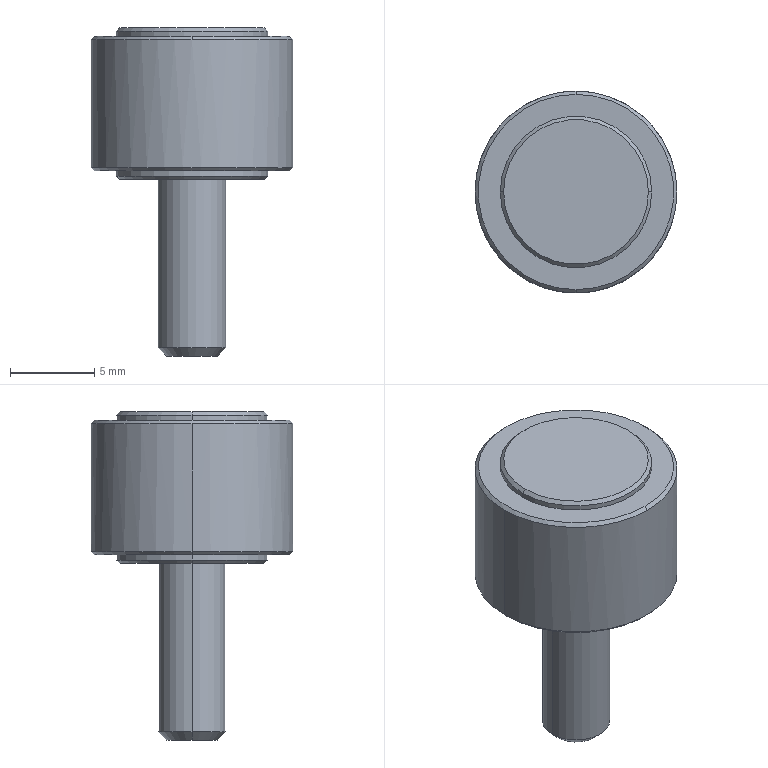Part | SolidWorks | features BaseBody 1 | 1 solid | 23 faces | box 12 x 12 x 19.5 mm | volume 1096 mm3 | cone 10 | cylinder 8 | plane 5 | commonest cylinder face diameters 9 x4 4 x2 12 x2
STEP:
#1=CARTESIAN_POINT('',(0.6764,-3.448,0.2));
#2=VERTEX_POINT('',#1);
#3=CARTESIAN_POINT('',(-11.324,-3.448,0.2));
#4=VERTEX_POINT('',#3);
#5=CARTESIAN_POINT('',(-5.324,-3.448,0.2));
#6=DIRECTION('',(0.,0.,1.));
#7=DIRECTION('',(1.,0.,0.));
#8=AXIS2_PLACEMENT_3D('',#5,#6,#7);
#9=CIRCLE('',#8,6.);
#10=EDGE_CURVE('',#2,#4,#9,.T.);
#11=ORIENTED_EDGE('',*,*,#10,.T.);
#12=CARTESIAN_POINT('',(-11.324,-3.448,7.8));
#13=VERTEX_POINT('',#12);
#14=CARTESIAN_POINT('',(-11.324,-3.448,0.));
#15=DIRECTION('',(0.,0.,1.));
#16=VECTOR('',#15,1000.);
#17=LINE('',#14,#16);
#18=EDGE_CURVE('',#4,#13,#17,.T.);
#19=ORIENTED_EDGE('',*,*,#18,.T.);
#20=CARTESIAN_POINT('',(-5.324,2.552,7.8));
#21=VERTEX_POINT('',#20);
#22=CARTESIAN_POINT('',(-5.324,-3.448,7.8));
#23=DIRECTION('',(0.,0.,-1.));
#24=DIRECTION('',(1.,0.,0.));
#25=AXIS2_PLACEMENT_3D('',#22,#23,#24);
#26=CIRCLE('',#25,6.);
#27=EDGE_CURVE('',#13,#21,#26,.T.);
#28=ORIENTED_EDGE('',*,*,#27,.T.);
#29=CARTESIAN_POINT('',(0.6764,-3.448,7.8));
#30=VERTEX_POINT('',#29);
#31=CARTESIAN_POINT('',(-5.324,-3.448,7.8));
#32=DIRECTION('',(0.,0.,-1.));
#33=DIRECTION('',(1.,0.,0.));
#34=AXIS2_PLACEMENT_3D('',#31,#32,#33);
#35=CIRCLE('',#34,6.);
#36=EDGE_CURVE('',#21,#30,#35,.T.);
#37=ORIENTED_EDGE('',*,*,#36,.T.);
#38=CARTESIAN_POINT('',(0.6764,-3.448,0.));
#39=DIRECTION('',(0.,0.,1.));
#40=VECTOR('',#39,1000.);
#41=LINE('',#38,#40);
#42=EDGE_CURVE('',#2,#30,#41,.T.);
#43=ORIENTED_EDGE('',*,*,#42,.F.);
#44=EDGE_LOOP('',(#11,#19,#28,#37,#43));
#45=FACE_OUTER_BOUND('',#44,.T.);
#46=CARTESIAN_POINT('',(-5.324,-3.448,0.));
#47=DIRECTION('',(0.,0.,1.));
#48=DIRECTION('',(1.,0.,0.));
#49=AXIS2_PLACEMENT_3D('',#46,#47,#48);
#50=CYLINDRICAL_SURFACE('',#49,6.);
#51=ADVANCED_FACE('',(#45),#50,.T.);
#52=CARTESIAN_POINT('',(0.4764,-3.448,0.));
#53=VERTEX_POINT('',#52);
#54=CARTESIAN_POINT('',(-11.124,-3.448,0.));
#55=VERTEX_POINT('',#54);
#56=CARTESIAN_POINT('',(-5.324,-3.448,0.));
#57=DIRECTION('',(0.,0.,1.));
#58=DIRECTION('',(1.,0.,0.));
#59=AXIS2_PLACEMENT_3D('',#56,#57,#58);
#60=CIRCLE('',#59,5.8);
#61=EDGE_CURVE('',#53,#55,#60,.T.);
#62=ORIENTED_EDGE('',*,*,#61,.T.);
#63=CARTESIAN_POINT('',(-11.324,-3.448,0.2));
#64=DIRECTION('',(-0.7071,0.,0.7071));
#65=VECTOR('',#64,1000.);
#66=LINE('',#63,#65);
#67=EDGE_CURVE('',#55,#4,#66,.T.);
#68=ORIENTED_EDGE('',*,*,#67,.T.);
#69=ORIENTED_EDGE('',*,*,#10,.F.);
#70=CARTESIAN_POINT('',(0.6764,-3.448,0.2));
#71=DIRECTION('',(0.7071,0.,0.7071));
#72=VECTOR('',#71,1000.);
#73=LINE('',#70,#72);
#74=EDGE_CURVE('',#53,#2,#73,.T.);
#75=ORIENTED_EDGE('',*,*,#74,.F.);
#76=EDGE_LOOP('',(#62,#68,#69,#75));
#77=FACE_OUTER_BOUND('',#76,.T.);
#78=CARTESIAN_POINT('',(-5.324,-3.448,0.2));
#79=DIRECTION('',(0.,0.,1.));
#80=DIRECTION('',(1.,0.,0.));
#81=AXIS2_PLACEMENT_3D('',#78,#79,#80);
#82=CONICAL_SURFACE('',#81,6.,0.7854);
#83=ADVANCED_FACE('',(#77),#82,.T.);
#84=CARTESIAN_POINT('',(-5.324,2.352,8.));
#85=VERTEX_POINT('',#84);
#86=CARTESIAN_POINT('',(-5.324,-9.248,8.));
#87=VERTEX_POINT('',#86);
#88=CARTESIAN_POINT('',(-5.324,-3.448,8.));
#89=DIRECTION('',(0.,0.,-1.));
#90=DIRECTION('',(0.,1.,0.));
#91=AXIS2_PLACEMENT_3D('',#88,#89,#90);
#92=CIRCLE('',#91,5.8);
#93=EDGE_CURVE('',#85,#87,#92,.T.);
#94=ORIENTED_EDGE('',*,*,#93,.T.);
#95=CARTESIAN_POINT('',(-5.324,-9.448,7.8));
#96=VERTEX_POINT('',#95);
#97=CARTESIAN_POINT('',(-5.324,-9.448,7.8));
#98=DIRECTION('',(0.,-0.7071,-0.7071));
#99=VECTOR('',#98,1000.);
#100=LINE('',#97,#99);
#101=EDGE_CURVE('',#87,#96,#100,.T.);
#102=ORIENTED_EDGE('',*,*,#101,.T.);
#103=CARTESIAN_POINT('',(-5.324,-3.448,7.8));
#104=DIRECTION('',(0.,0.,-1.));
#105=DIRECTION('',(1.,0.,0.));
#106=AXIS2_PLACEMENT_3D('',#103,#104,#105);
#107=CIRCLE('',#106,6.);
#108=EDGE_CURVE('',#30,#96,#107,.T.);
#109=ORIENTED_EDGE('',*,*,#108,.F.);
#110=ORIENTED_EDGE('',*,*,#36,.F.);
#111=CARTESIAN_POINT('',(-5.324,2.552,7.8));
#112=DIRECTION('',(0.,0.7071,-0.7071));
#113=VECTOR('',#112,1000.);
#114=LINE('',#111,#113);
#115=EDGE_CURVE('',#85,#21,#114,.T.);
#116=ORIENTED_EDGE('',*,*,#115,.F.);
#117=EDGE_LOOP('',(#94,#102,#109,#110,#116));
#118=FACE_OUTER_BOUND('',#117,.T.);
#119=CARTESIAN_POINT('',(-5.324,-3.448,7.8));
#120=DIRECTION('',(0.,0.,-1.));
#121=DIRECTION('',(0.,1.,0.));
#122=AXIS2_PLACEMENT_3D('',#119,#120,#121);
#123=CONICAL_SURFACE('',#122,6.,0.7854);
#124=ADVANCED_FACE('',(#118),#123,.T.);
#125=CARTESIAN_POINT('',(-0.8236,-3.448,0.));
#126=VERTEX_POINT('',#125);
#127=CARTESIAN_POINT('',(-9.824,-3.448,0.));
#128=VERTEX_POINT('',#127);
#129=CARTESIAN_POINT('',(-5.324,-3.448,0.));
#130=DIRECTION('',(0.,0.,1.));
#131=DIRECTION('',(-1.,0.,0.));
#132=AXIS2_PLACEMENT_3D('',#129,#130,#131);
#133=CIRCLE('',#132,4.5);
#134=EDGE_CURVE('',#126,#128,#133,.T.);
#135=ORIENTED_EDGE('',*,*,#134,.F.);
#136=CARTESIAN_POINT('',(-0.8236,-3.448,-0.3));
#137=VERTEX_POINT('',#136);
#138=CARTESIAN_POINT('',(-0.8236,-3.448,0.));
#139=DIRECTION('',(0.,0.,-1.));
#140=VECTOR('',#139,1000.);
#141=LINE('',#138,#140);
#142=EDGE_CURVE('',#126,#137,#141,.T.);
#143=ORIENTED_EDGE('',*,*,#142,.T.);
#144=CARTESIAN_POINT('',(-9.824,-3.448,-0.3));
#145=VERTEX_POINT('',#144);
#146=CARTESIAN_POINT('',(-5.324,-3.448,-0.3));
#147=DIRECTION('',(0.,0.,1.));
#148=DIRECTION('',(-1.,0.,0.));
#149=AXIS2_PLACEMENT_3D('',#146,#147,#148);
#150=CIRCLE('',#149,4.5);
#151=EDGE_CURVE('',#137,#145,#150,.T.);
#152=ORIENTED_EDGE('',*,*,#151,.T.);
#153=CARTESIAN_POINT('',(-9.824,-3.448,0.));
#154=DIRECTION('',(0.,0.,-1.));
#155=VECTOR('',#154,1000.);
#156=LINE('',#153,#155);
#157=EDGE_CURVE('',#128,#145,#156,.T.);
#158=ORIENTED_EDGE('',*,*,#157,.F.);
#159=EDGE_LOOP('',(#135,#143,#152,#158));
#160=FACE_OUTER_BOUND('',#159,.T.);
#161=CARTESIAN_POINT('',(-5.324,-3.448,0.));
#162=DIRECTION('',(0.,0.,-1.));
#163=DIRECTION('',(-1.,0.,0.));
#164=AXIS2_PLACEMENT_3D('',#161,#162,#163);
#165=CYLINDRICAL_SURFACE('',#164,4.5);
#166=ADVANCED_FACE('',(#160),#165,.T.);
#167=CARTESIAN_POINT('',(-0.8236,-3.448,8.));
#168=VERTEX_POINT('',#167);
#169=CARTESIAN_POINT('',(-9.824,-3.448,8.));
#170=VERTEX_POINT('',#169);
#171=CARTESIAN_POINT('',(-5.324,-3.448,8.));
#172=DIRECTION('',(0.,0.,1.));
#173=DIRECTION('',(1.,0.,0.));
#174=AXIS2_PLACEMENT_3D('',#171,#172,#173);
#175=CIRCLE('',#174,4.5);
#176=EDGE_CURVE('',#168,#170,#175,.T.);
#177=ORIENTED_EDGE('',*,*,#176,.T.);
#178=CARTESIAN_POINT('',(-9.824,-3.448,8.3));
#179=VERTEX_POINT('',#178);
#180=CARTESIAN_POINT('',(-9.824,-3.448,8.));
#181=DIRECTION('',(0.,0.,1.));
#182=VECTOR('',#181,1000.);
#183=LINE('',#180,#182);
#184=EDGE_CURVE('',#170,#179,#183,.T.);
#185=ORIENTED_EDGE('',*,*,#184,.T.);
#186=CARTESIAN_POINT('',(-0.8236,-3.448,8.3));
#187=VERTEX_POINT('',#186);
#188=CARTESIAN_POINT('',(-5.324,-3.448,8.3));
#189=DIRECTION('',(0.,0.,-1.));
#190=DIRECTION('',(1.,0.,0.));
#191=AXIS2_PLACEMENT_3D('',#188,#189,#190);
#192=CIRCLE('',#191,4.5);
#193=EDGE_CURVE('',#179,#187,#192,.T.);
#194=ORIENTED_EDGE('',*,*,#193,.T.);
#195=CARTESIAN_POINT('',(-0.8236,-3.448,8.));
#196=DIRECTION('',(0.,0.,1.));
#197=VECTOR('',#196,1000.);
#198=LINE('',#195,#197);
#199=EDGE_CURVE('',#168,#187,#198,.T.);
#200=ORIENTED_EDGE('',*,*,#199,.F.);
#201=EDGE_LOOP('',(#177,#185,#194,#200));
#202=FACE_OUTER_BOUND('',#201,.T.);
#203=CARTESIAN_POINT('',(-5.324,-3.448,8.));
#204=DIRECTION('',(0.,0.,1.));
#205=DIRECTION('',(1.,0.,0.));
#206=AXIS2_PLACEMENT_3D('',#203,#204,#205);
#207=CYLINDRICAL_SURFACE('',#206,4.5);
#208=ADVANCED_FACE('',(#202),#207,.T.);
#209=CARTESIAN_POINT('',(-1.024,-3.448,-0.5));
#210=VERTEX_POINT('',#209);
#211=CARTESIAN_POINT('',(-9.624,-3.448,-0.5));
#212=VERTEX_POINT('',#211);
#213=CARTESIAN_POINT('',(-5.324,-3.448,-0.5));
#214=DIRECTION('',(0.,0.,1.));
#215=DIRECTION('',(1.,0.,0.));
#216=AXIS2_PLACEMENT_3D('',#213,#214,#215);
#217=CIRCLE('',#216,4.3);
#218=EDGE_CURVE('',#210,#212,#217,.T.);
#219=ORIENTED_EDGE('',*,*,#218,.T.);
#220=CARTESIAN_POINT('',(-9.824,-3.448,-0.3));
#221=DIRECTION('',(-0.7071,0.,0.7071));
#222=VECTOR('',#221,1000.);
#223=LINE('',#220,#222);
#224=EDGE_CURVE('',#212,#145,#223,.T.);
#225=ORIENTED_EDGE('',*,*,#224,.T.);
#226=ORIENTED_EDGE('',*,*,#151,.F.);
#227=CARTESIAN_POINT('',(-0.8236,-3.448,-0.3));
#228=DIRECTION('',(0.7071,0.,0.7071));
#229=VECTOR('',#228,1000.);
#230=LINE('',#227,#229);
#231=EDGE_CURVE('',#210,#137,#230,.T.);
#232=ORIENTED_EDGE('',*,*,#231,.F.);
#233=EDGE_LOOP('',(#219,#225,#226,#232));
#234=FACE_OUTER_BOUND('',#233,.T.);
#235=CARTESIAN_POINT('',(-5.324,-3.448,-0.3));
#236=DIRECTION('',(0.,0.,1.));
#237=DIRECTION('',(1.,0.,0.));
#238=AXIS2_PLACEMENT_3D('',#235,#236,#237);
#239=CONICAL_SURFACE('',#238,4.5,0.7854);
#240=ADVANCED_FACE('',(#234),#239,.T.);
#241=CARTESIAN_POINT('',(-9.624,-3.448,8.5));
#242=VERTEX_POINT('',#241);
#243=CARTESIAN_POINT('',(-1.024,-3.448,8.5));
#244=VERTEX_POINT('',#243);
#245=CARTESIAN_POINT('',(-5.324,-3.448,8.5));
#246=DIRECTION('',(0.,0.,-1.));
#247=DIRECTION('',(-1.,0.,0.));
#248=AXIS2_PLACEMENT_3D('',#245,#246,#247);
#249=CIRCLE('',#248,4.3);
#250=EDGE_CURVE('',#242,#244,#249,.T.);
#251=ORIENTED_EDGE('',*,*,#250,.T.);
#252=CARTESIAN_POINT('',(-0.8236,-3.448,8.3));
#253=DIRECTION('',(0.7071,0.,-0.7071));
#254=VECTOR('',#253,1000.);
#255=LINE('',#252,#254);
#256=EDGE_CURVE('',#244,#187,#255,.T.);
#257=ORIENTED_EDGE('',*,*,#256,.T.);
#258=ORIENTED_EDGE('',*,*,#193,.F.);
#259=CARTESIAN_POINT('',(-9.824,-3.448,8.3));
#260=DIRECTION('',(-0.7071,0.,-0.7071));
#261=VECTOR('',#260,1000.);
#262=LINE('',#259,#261);
#263=EDGE_CURVE('',#242,#179,#262,.T.);
#264=ORIENTED_EDGE('',*,*,#263,.F.);
#265=EDGE_LOOP('',(#251,#257,#258,#264));
#266=FACE_OUTER_BOUND('',#265,.T.);
#267=CARTESIAN_POINT('',(-5.324,-3.448,8.3));
#268=DIRECTION('',(0.,0.,-1.));
#269=DIRECTION('',(-1.,0.,0.));
#270=AXIS2_PLACEMENT_3D('',#267,#268,#269);
#271=CONICAL_SURFACE('',#270,4.5,0.7854);
#272=ADVANCED_FACE('',(#266),#271,.T.);
#273=CARTESIAN_POINT('',(-7.324,-3.448,-0.5));
#274=VERTEX_POINT('',#273);
#275=CARTESIAN_POINT('',(-3.324,-3.448,-0.5));
#276=VERTEX_POINT('',#275);
#277=CARTESIAN_POINT('',(-5.324,-3.448,-0.5));
#278=DIRECTION('',(0.,0.,-1.));
#279=DIRECTION('',(-1.,0.,0.));
#280=AXIS2_PLACEMENT_3D('',#277,#278,#279);
#281=CIRCLE('',#280,2.);
#282=EDGE_CURVE('',#274,#276,#281,.T.);
#283=ORIENTED_EDGE('',*,*,#282,.T.);
#284=CARTESIAN_POINT('',(-3.324,-3.448,-10.5));
#285=VERTEX_POINT('',#284);
#286=CARTESIAN_POINT('',(-3.324,-3.448,-0.5));
#287=DIRECTION('',(0.,0.,-1.));
#288=VECTOR('',#287,1000.);
#289=LINE('',#286,#288);
#290=EDGE_CURVE('',#276,#285,#289,.T.);
#291=ORIENTED_EDGE('',*,*,#290,.T.);
#292=CARTESIAN_POINT('',(-7.324,-3.448,-10.5));
#293=VERTEX_POINT('',#292);
#294=CARTESIAN_POINT('',(-5.324,-3.448,-10.5));
#295=DIRECTION('',(0.,0.,1.));
#296=DIRECTION('',(-1.,0.,0.));
#297=AXIS2_PLACEMENT_3D('',#294,#295,#296);
#298=CIRCLE('',#297,2.);
#299=EDGE_CURVE('',#285,#293,#298,.T.);
#300=ORIENTED_EDGE('',*,*,#299,.T.);
#301=CARTESIAN_POINT('',(-7.324,-3.448,-0.5));
#302=DIRECTION('',(0.,0.,-1.));
#303=VECTOR('',#302,1000.);
#304=LINE('',#301,#303);
#305=EDGE_CURVE('',#274,#293,#304,.T.);
#306=ORIENTED_EDGE('',*,*,#305,.F.);
#307=EDGE_LOOP('',(#283,#291,#300,#306));
#308=FACE_OUTER_BOUND('',#307,.T.);
#309=CARTESIAN_POINT('',(-5.324,-3.448,-0.5));
#310=DIRECTION('',(0.,0.,-1.));
#311=DIRECTION('',(-1.,0.,0.));
#312=AXIS2_PLACEMENT_3D('',#309,#310,#311);
#313=CYLINDRICAL_SURFACE('',#312,2.);
#314=ADVANCED_FACE('',(#308),#313,.T.);
#315=CARTESIAN_POINT('',(-3.824,-3.448,-11.));
#316=VERTEX_POINT('',#315);
#317=CARTESIAN_POINT('',(-6.824,-3.448,-11.));
#318=VERTEX_POINT('',#317);
#319=CARTESIAN_POINT('',(-5.324,-3.448,-11.));
#320=DIRECTION('',(0.,0.,1.));
#321=DIRECTION('',(1.,0.,0.));
#322=AXIS2_PLACEMENT_3D('',#319,#320,#321);
#323=CIRCLE('',#322,1.5);
#324=EDGE_CURVE('',#316,#318,#323,.T.);
#325=ORIENTED_EDGE('',*,*,#324,.T.);
#326=CARTESIAN_POINT('',(-7.324,-3.448,-10.5));
#327=DIRECTION('',(-0.7071,0.,0.7071));
#328=VECTOR('',#327,1000.);
#329=LINE('',#326,#328);
#330=EDGE_CURVE('',#318,#293,#329,.T.);
#331=ORIENTED_EDGE('',*,*,#330,.T.);
#332=ORIENTED_EDGE('',*,*,#299,.F.);
#333=CARTESIAN_POINT('',(-3.324,-3.448,-10.5));
#334=DIRECTION('',(0.7071,0.,0.7071));
#335=VECTOR('',#334,1000.);
#336=LINE('',#333,#335);
#337=EDGE_CURVE('',#316,#285,#336,.T.);
#338=ORIENTED_EDGE('',*,*,#337,.F.);
#339=EDGE_LOOP('',(#325,#331,#332,#338));
#340=FACE_OUTER_BOUND('',#339,.T.);
#341=CARTESIAN_POINT('',(-5.324,-3.448,-10.5));
#342=DIRECTION('',(0.,0.,1.));
#343=DIRECTION('',(1.,0.,0.));
#344=AXIS2_PLACEMENT_3D('',#341,#342,#343);
#345=CONICAL_SURFACE('',#344,2.,0.7854);
#346=ADVANCED_FACE('',(#340),#345,.T.);
#347=ORIENTED_EDGE('',*,*,#18,.F.);
#348=CARTESIAN_POINT('',(-5.324,-3.448,0.2));
#349=DIRECTION('',(0.,0.,1.));
#350=DIRECTION('',(1.,0.,0.));
#351=AXIS2_PLACEMENT_3D('',#348,#349,#350);
#352=CIRCLE('',#351,6.);
#353=EDGE_CURVE('',#4,#2,#352,.T.);
#354=ORIENTED_EDGE('',*,*,#353,.T.);
#355=ORIENTED_EDGE('',*,*,#42,.T.);
#356=ORIENTED_EDGE('',*,*,#108,.T.);
#357=CARTESIAN_POINT('',(-5.324,-3.448,7.8));
#358=DIRECTION('',(0.,0.,-1.));
#359=DIRECTION('',(1.,0.,0.));
#360=AXIS2_PLACEMENT_3D('',#357,#358,#359);
#361=CIRCLE('',#360,6.);
#362=EDGE_CURVE('',#96,#13,#361,.T.);
#363=ORIENTED_EDGE('',*,*,#362,.T.);
#364=EDGE_LOOP('',(#347,#354,#355,#356,#363));
#365=FACE_OUTER_BOUND('',#364,.T.);
#366=CARTESIAN_POINT('',(-5.324,-3.448,0.));
#367=DIRECTION('',(0.,0.,1.));
#368=DIRECTION('',(1.,0.,0.));
#369=AXIS2_PLACEMENT_3D('',#366,#367,#368);
#370=CYLINDRICAL_SURFACE('',#369,6.);
#371=ADVANCED_FACE('',(#365),#370,.T.);
#372=ORIENTED_EDGE('',*,*,#67,.F.);
#373=CARTESIAN_POINT('',(-5.324,-3.448,0.));
#374=DIRECTION('',(0.,0.,1.));
#375=DIRECTION('',(1.,0.,0.));
#376=AXIS2_PLACEMENT_3D('',#373,#374,#375);
#377=CIRCLE('',#376,5.8);
#378=EDGE_CURVE('',#55,#53,#377,.T.);
#379=ORIENTED_EDGE('',*,*,#378,.T.);
#380=ORIENTED_EDGE('',*,*,#74,.T.);
#381=ORIENTED_EDGE('',*,*,#353,.F.);
#382=EDGE_LOOP('',(#372,#379,#380,#381));
#383=FACE_OUTER_BOUND('',#382,.T.);
#384=CARTESIAN_POINT('',(-5.324,-3.448,0.2));
#385=DIRECTION('',(0.,0.,1.));
#386=DIRECTION('',(1.,0.,0.));
#387=AXIS2_PLACEMENT_3D('',#384,#385,#386);
#388=CONICAL_SURFACE('',#387,6.,0.7854);
#389=ADVANCED_FACE('',(#383),#388,.T.);
#390=ORIENTED_EDGE('',*,*,#101,.F.);
#391=CARTESIAN_POINT('',(-5.324,-3.448,8.));
#392=DIRECTION('',(0.,0.,-1.));
#393=DIRECTION('',(0.,1.,0.));
#394=AXIS2_PLACEMENT_3D('',#391,#392,#393);
#395=CIRCLE('',#394,5.8);
#396=EDGE_CURVE('',#87,#85,#395,.T.);
#397=ORIENTED_EDGE('',*,*,#396,.T.);
#398=ORIENTED_EDGE('',*,*,#115,.T.);
#399=ORIENTED_EDGE('',*,*,#27,.F.);
#400=ORIENTED_EDGE('',*,*,#362,.F.);
#401=EDGE_LOOP('',(#390,#397,#398,#399,#400));
#402=FACE_OUTER_BOUND('',#401,.T.);
#403=CARTESIAN_POINT('',(-5.324,-3.448,7.8));
#404=DIRECTION('',(0.,0.,-1.));
#405=DIRECTION('',(0.,1.,0.));
#406=AXIS2_PLACEMENT_3D('',#403,#404,#405);
#407=CONICAL_SURFACE('',#406,6.,0.7854);
#408=ADVANCED_FACE('',(#402),#407,.T.);
#409=CARTESIAN_POINT('',(-5.324,-3.448,0.));
#410=DIRECTION('',(0.,0.,1.));
#411=DIRECTION('',(-1.,0.,0.));
#412=AXIS2_PLACEMENT_3D('',#409,#410,#411);
#413=CIRCLE('',#412,4.5);
#414=EDGE_CURVE('',#128,#126,#413,.T.);
#415=ORIENTED_EDGE('',*,*,#414,.T.);
#416=ORIENTED_EDGE('',*,*,#134,.T.);
#417=EDGE_LOOP('',(#415,#416));
#418=FACE_BOUND('',#417,.T.);
#419=ORIENTED_EDGE('',*,*,#61,.F.);
#420=ORIENTED_EDGE('',*,*,#378,.F.);
#421=EDGE_LOOP('',(#419,#420));
#422=FACE_OUTER_BOUND('',#421,.T.);
#423=CARTESIAN_POINT('',(-5.324,-3.448,0.));
#424=DIRECTION('',(0.,0.,-1.));
#425=DIRECTION('',(-1.,0.,0.));
#426=AXIS2_PLACEMENT_3D('',#423,#424,#425);
#427=PLANE('',#426);
#428=ADVANCED_FACE('',(#418,#422),#427,.T.);
#429=ORIENTED_EDGE('',*,*,#176,.F.);
#430=CARTESIAN_POINT('',(-5.324,-3.448,8.));
#431=DIRECTION('',(0.,0.,1.));
#432=DIRECTION('',(1.,0.,0.));
#433=AXIS2_PLACEMENT_3D('',#430,#431,#432);
#434=CIRCLE('',#433,4.5);
#435=EDGE_CURVE('',#170,#168,#434,.T.);
#436=ORIENTED_EDGE('',*,*,#435,.F.);
#437=EDGE_LOOP('',(#429,#436));
#438=FACE_BOUND('',#437,.T.);
#439=ORIENTED_EDGE('',*,*,#93,.F.);
#440=ORIENTED_EDGE('',*,*,#396,.F.);
#441=EDGE_LOOP('',(#439,#440));
#442=FACE_OUTER_BOUND('',#441,.T.);
#443=CARTESIAN_POINT('',(-5.324,-3.448,8.));
#444=DIRECTION('',(0.,0.,-1.));
#445=DIRECTION('',(-1.,0.,0.));
#446=AXIS2_PLACEMENT_3D('',#443,#444,#445);
#447=PLANE('',#446);
#448=ADVANCED_FACE('',(#438,#442),#447,.F.);
#449=ORIENTED_EDGE('',*,*,#142,.F.);
#450=ORIENTED_EDGE('',*,*,#414,.F.);
#451=ORIENTED_EDGE('',*,*,#157,.T.);
#452=CARTESIAN_POINT('',(-5.324,-3.448,-0.3));
#453=DIRECTION('',(0.,0.,1.));
#454=DIRECTION('',(-1.,0.,0.));
#455=AXIS2_PLACEMENT_3D('',#452,#453,#454);
#456=CIRCLE('',#455,4.5);
#457=EDGE_CURVE('',#145,#137,#456,.T.);
#458=ORIENTED_EDGE('',*,*,#457,.T.);
#459=EDGE_LOOP('',(#449,#450,#451,#458));
#460=FACE_OUTER_BOUND('',#459,.T.);
#461=CARTESIAN_POINT('',(-5.324,-3.448,0.));
#462=DIRECTION('',(0.,0.,-1.));
#463=DIRECTION('',(-1.,0.,0.));
#464=AXIS2_PLACEMENT_3D('',#461,#462,#463);
#465=CYLINDRICAL_SURFACE('',#464,4.5);
#466=ADVANCED_FACE('',(#460),#465,.T.);
#467=ORIENTED_EDGE('',*,*,#184,.F.);
#468=ORIENTED_EDGE('',*,*,#435,.T.);
#469=ORIENTED_EDGE('',*,*,#199,.T.);
#470=CARTESIAN_POINT('',(-5.324,-3.448,8.3));
#471=DIRECTION('',(0.,0.,-1.));
#472=DIRECTION('',(1.,0.,0.));
#473=AXIS2_PLACEMENT_3D('',#470,#471,#472);
#474=CIRCLE('',#473,4.5);
#475=EDGE_CURVE('',#187,#179,#474,.T.);
#476=ORIENTED_EDGE('',*,*,#475,.T.);
#477=EDGE_LOOP('',(#467,#468,#469,#476));
#478=FACE_OUTER_BOUND('',#477,.T.);
#479=CARTESIAN_POINT('',(-5.324,-3.448,8.));
#480=DIRECTION('',(0.,0.,1.));
#481=DIRECTION('',(1.,0.,0.));
#482=AXIS2_PLACEMENT_3D('',#479,#480,#481);
#483=CYLINDRICAL_SURFACE('',#482,4.5);
#484=ADVANCED_FACE('',(#478),#483,.T.);
#485=ORIENTED_EDGE('',*,*,#224,.F.);
#486=CARTESIAN_POINT('',(-5.324,-3.448,-0.5));
#487=DIRECTION('',(0.,0.,1.));
#488=DIRECTION('',(1.,0.,0.));
#489=AXIS2_PLACEMENT_3D('',#486,#487,#488);
#490=CIRCLE('',#489,4.3);
#491=EDGE_CURVE('',#212,#210,#490,.T.);
#492=ORIENTED_EDGE('',*,*,#491,.T.);
#493=ORIENTED_EDGE('',*,*,#231,.T.);
#494=ORIENTED_EDGE('',*,*,#457,.F.);
#495=EDGE_LOOP('',(#485,#492,#493,#494));
#496=FACE_OUTER_BOUND('',#495,.T.);
#497=CARTESIAN_POINT('',(-5.324,-3.448,-0.3));
#498=DIRECTION('',(0.,0.,1.));
#499=DIRECTION('',(1.,0.,0.));
#500=AXIS2_PLACEMENT_3D('',#497,#498,#499);
#501=CONICAL_SURFACE('',#500,4.5,0.7854);
#502=ADVANCED_FACE('',(#496),#501,.T.);
#503=ORIENTED_EDGE('',*,*,#256,.F.);
#504=CARTESIAN_POINT('',(-5.324,-3.448,8.5));
#505=DIRECTION('',(0.,0.,-1.));
#506=DIRECTION('',(-1.,0.,0.));
#507=AXIS2_PLACEMENT_3D('',#504,#505,#506);
#508=CIRCLE('',#507,4.3);
#509=EDGE_CURVE('',#244,#242,#508,.T.);
#510=ORIENTED_EDGE('',*,*,#509,.T.);
#511=ORIENTED_EDGE('',*,*,#263,.T.);
#512=ORIENTED_EDGE('',*,*,#475,.F.);
#513=EDGE_LOOP('',(#503,#510,#511,#512));
#514=FACE_OUTER_BOUND('',#513,.T.);
#515=CARTESIAN_POINT('',(-5.324,-3.448,8.3));
#516=DIRECTION('',(0.,0.,-1.));
#517=DIRECTION('',(-1.,0.,0.));
#518=AXIS2_PLACEMENT_3D('',#515,#516,#517);
#519=CONICAL_SURFACE('',#518,4.5,0.7854);
#520=ADVANCED_FACE('',(#514),#519,.T.);
#521=ORIENTED_EDGE('',*,*,#282,.F.);
#522=CARTESIAN_POINT('',(-5.324,-3.448,-0.5));
#523=DIRECTION('',(0.,0.,-1.));
#524=DIRECTION('',(-1.,0.,0.));
#525=AXIS2_PLACEMENT_3D('',#522,#523,#524);
#526=CIRCLE('',#525,2.);
#527=EDGE_CURVE('',#276,#274,#526,.T.);
#528=ORIENTED_EDGE('',*,*,#527,.F.);
#529=EDGE_LOOP('',(#521,#528));
#530=FACE_BOUND('',#529,.T.);
#531=ORIENTED_EDGE('',*,*,#218,.F.);
#532=ORIENTED_EDGE('',*,*,#491,.F.);
#533=EDGE_LOOP('',(#531,#532));
#534=FACE_OUTER_BOUND('',#533,.T.);
#535=CARTESIAN_POINT('',(-5.324,-3.448,-0.5));
#536=DIRECTION('',(0.,0.,1.));
#537=DIRECTION('',(1.,0.,0.));
#538=AXIS2_PLACEMENT_3D('',#535,#536,#537);
#539=PLANE('',#538);
#540=ADVANCED_FACE('',(#530,#534),#539,.F.);
#541=ORIENTED_EDGE('',*,*,#250,.F.);
#542=ORIENTED_EDGE('',*,*,#509,.F.);
#543=EDGE_LOOP('',(#541,#542));
#544=FACE_OUTER_BOUND('',#543,.T.);
#545=CARTESIAN_POINT('',(-5.324,-3.448,8.5));
#546=DIRECTION('',(0.,0.,-1.));
#547=DIRECTION('',(-1.,0.,0.));
#548=AXIS2_PLACEMENT_3D('',#545,#546,#547);
#549=PLANE('',#548);
#550=ADVANCED_FACE('',(#544),#549,.F.);
#551=ORIENTED_EDGE('',*,*,#290,.F.);
#552=ORIENTED_EDGE('',*,*,#527,.T.);
#553=ORIENTED_EDGE('',*,*,#305,.T.);
#554=CARTESIAN_POINT('',(-5.324,-3.448,-10.5));
#555=DIRECTION('',(0.,0.,1.));
#556=DIRECTION('',(-1.,0.,0.));
#557=AXIS2_PLACEMENT_3D('',#554,#555,#556);
#558=CIRCLE('',#557,2.);
#559=EDGE_CURVE('',#293,#285,#558,.T.);
#560=ORIENTED_EDGE('',*,*,#559,.T.);
#561=EDGE_LOOP('',(#551,#552,#553,#560));
#562=FACE_OUTER_BOUND('',#561,.T.);
#563=CARTESIAN_POINT('',(-5.324,-3.448,-0.5));
#564=DIRECTION('',(0.,0.,-1.));
#565=DIRECTION('',(-1.,0.,0.));
#566=AXIS2_PLACEMENT_3D('',#563,#564,#565);
#567=CYLINDRICAL_SURFACE('',#566,2.);
#568=ADVANCED_FACE('',(#562),#567,.T.);
#569=ORIENTED_EDGE('',*,*,#330,.F.);
#570=CARTESIAN_POINT('',(-5.324,-3.448,-11.));
#571=DIRECTION('',(0.,0.,1.));
#572=DIRECTION('',(1.,0.,0.));
#573=AXIS2_PLACEMENT_3D('',#570,#571,#572);
#574=CIRCLE('',#573,1.5);
#575=EDGE_CURVE('',#318,#316,#574,.T.);
#576=ORIENTED_EDGE('',*,*,#575,.T.);
#577=ORIENTED_EDGE('',*,*,#337,.T.);
#578=ORIENTED_EDGE('',*,*,#559,.F.);
#579=EDGE_LOOP('',(#569,#576,#577,#578));
#580=FACE_OUTER_BOUND('',#579,.T.);
#581=CARTESIAN_POINT('',(-5.324,-3.448,-10.5));
#582=DIRECTION('',(0.,0.,1.));
#583=DIRECTION('',(1.,0.,0.));
#584=AXIS2_PLACEMENT_3D('',#581,#582,#583);
#585=CONICAL_SURFACE('',#584,2.,0.7854);
#586=ADVANCED_FACE('',(#580),#585,.T.);
#587=ORIENTED_EDGE('',*,*,#324,.F.);
#588=ORIENTED_EDGE('',*,*,#575,.F.);
#589=EDGE_LOOP('',(#587,#588));
#590=FACE_OUTER_BOUND('',#589,.T.);
#591=CARTESIAN_POINT('',(-5.324,-3.448,-11.));
#592=DIRECTION('',(0.,0.,1.));
#593=DIRECTION('',(1.,0.,0.));
#594=AXIS2_PLACEMENT_3D('',#591,#592,#593);
#595=PLANE('',#594);
#596=ADVANCED_FACE('',(#590),#595,.F.);
#597=CLOSED_SHELL('',(#51,#83,#124,#166,#208,#240,#272,#314,#346,#371,#389,#408,#428,#448,#466,#484,#502,#520,#540,#550,#568,#586,#596));
#598=MANIFOLD_SOLID_BREP('',#597);
#599=CARTESIAN_POINT('',(0.,0.,0.));
#600=DIRECTION('',(0.,0.,1.));
#601=DIRECTION('',(1.,0.,0.));
#602=AXIS2_PLACEMENT_3D('',#599,#600,#601);
#603=(LENGTH_UNIT()NAMED_UNIT(*)SI_UNIT(.MILLI.,.METRE.));
#604=UNCERTAINTY_MEASURE_WITH_UNIT(LENGTH_MEASURE(0.00001),#603,'','');
#605=(NAMED_UNIT(*)PLANE_ANGLE_UNIT()SI_UNIT($,.RADIAN.));
#606=(NAMED_UNIT(*)SI_UNIT($,.STERADIAN.)SOLID_ANGLE_UNIT());
#607=(GEOMETRIC_REPRESENTATION_CONTEXT(3)GLOBAL_UNCERTAINTY_ASSIGNED_CONTEXT((#604))GLOBAL_UNIT_ASSIGNED_CONTEXT((#603,#605,#606))REPRESENTATION_CONTEXT('',''));
#608=ADVANCED_BREP_SHAPE_REPRESENTATION('',(#598,#602),#607);